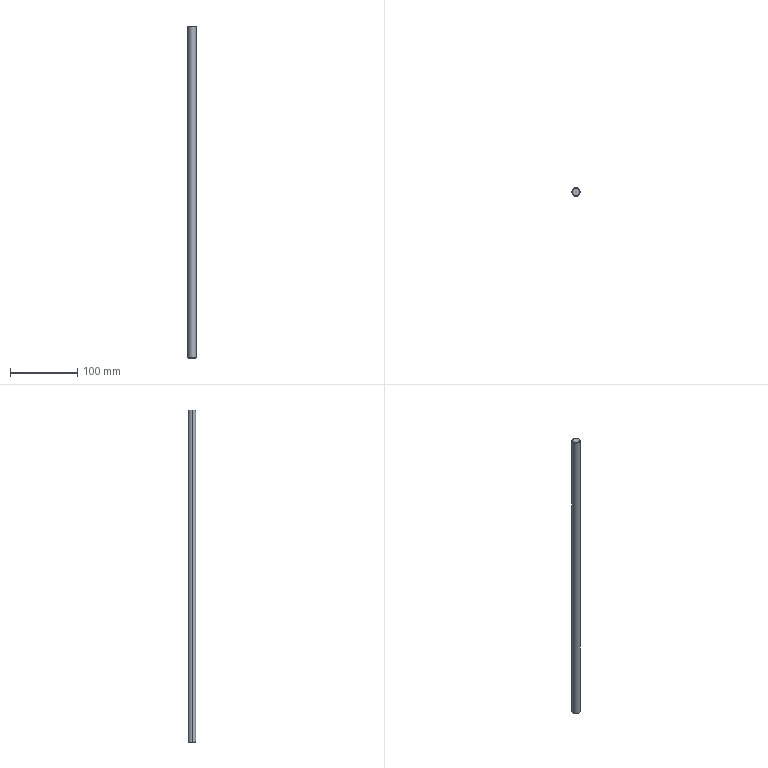Part | STEP file | 0230_011_SSFJ12-495 | 1 solid | 8 faces | box 12 x 12 x 495 mm | volume 55974 mm3 | cone 4 | cylinder 2 | plane 2 | commonest cylinder face diameters 12 x2
STEP:
#1=CARTESIAN_POINT('',(0.,0.,0.));
#2=DIRECTION('',(0.,0.,1.));
#3=DIRECTION('',(1.,0.,0.));
#4=AXIS2_PLACEMENT_3D('',#1,#2,#3);
#5=CARTESIAN_POINT('',(5.5,0.,495.));
#6=VERTEX_POINT('',#5);
#7=CARTESIAN_POINT('',(-5.5,0.,495.));
#8=VERTEX_POINT('',#7);
#9=CARTESIAN_POINT('',(0.,0.,495.));
#10=DIRECTION('',(0.,0.,1.));
#11=DIRECTION('',(1.,0.,0.));
#12=AXIS2_PLACEMENT_3D('',#9,#10,#11);
#13=CIRCLE('',#12,5.5);
#14=CARTESIAN_POINT('',(0.,0.,495.));
#15=DIRECTION('',(0.,0.,-1.));
#16=DIRECTION('',(-1.,0.,0.));
#17=AXIS2_PLACEMENT_3D('',#14,#15,#16);
#18=CONICAL_SURFACE('',#17,5.5,0.7854);
#19=CARTESIAN_POINT('',(3.142,0.));
#20=DIRECTION('',(-1.,0.));
#21=VECTOR('',#20,1.);
#22=LINE('',#19,#21);
#23=(GEOMETRIC_REPRESENTATION_CONTEXT(2)PARAMETRIC_REPRESENTATION_CONTEXT()REPRESENTATION_CONTEXT('',''));
#24=DEFINITIONAL_REPRESENTATION('',(#22),#23);
#25=PCURVE('',#18,#24);
#26=CARTESIAN_POINT('',(0.,0.,495.));
#27=DIRECTION('',(0.,0.,1.));
#28=DIRECTION('',(1.,0.,0.));
#29=AXIS2_PLACEMENT_3D('',#26,#27,#28);
#30=PLANE('',#29);
#31=CARTESIAN_POINT('',(0.,0.));
#32=DIRECTION('',(1.,0.));
#33=AXIS2_PLACEMENT_2D('',#31,#32);
#34=CIRCLE('',#33,5.5);
#35=(GEOMETRIC_REPRESENTATION_CONTEXT(2)PARAMETRIC_REPRESENTATION_CONTEXT()REPRESENTATION_CONTEXT('',''));
#36=DEFINITIONAL_REPRESENTATION('',(#34),#35);
#37=PCURVE('',#30,#36);
#38=SURFACE_CURVE('',#13,(#25,#37),.PCURVE_S1.);
#39=EDGE_CURVE('',#6,#8,#38,.T.);
#40=ORIENTED_EDGE('',*,*,#39,.F.);
#41=CARTESIAN_POINT('',(6.,0.,494.5));
#42=VERTEX_POINT('',#41);
#43=CARTESIAN_POINT('',(5.5,0.,495.));
#44=DIRECTION('',(0.7071,0.,-0.7071));
#45=VECTOR('',#44,1.);
#46=LINE('',#43,#45);
#47=CARTESIAN_POINT('',(3.142,0.));
#48=DIRECTION('',(0.,1.));
#49=VECTOR('',#48,1.);
#50=LINE('',#47,#49);
#51=(GEOMETRIC_REPRESENTATION_CONTEXT(2)PARAMETRIC_REPRESENTATION_CONTEXT()REPRESENTATION_CONTEXT('',''));
#52=DEFINITIONAL_REPRESENTATION('',(#50),#51);
#53=PCURVE('',#18,#52);
#54=CARTESIAN_POINT('',(0.,0.,495.));
#55=DIRECTION('',(0.,0.,-1.));
#56=DIRECTION('',(-1.,0.,0.));
#57=AXIS2_PLACEMENT_3D('',#54,#55,#56);
#58=CONICAL_SURFACE('',#57,5.5,0.7854);
#59=CARTESIAN_POINT('',(3.142,0.));
#60=DIRECTION('',(0.,1.));
#61=VECTOR('',#60,1.);
#62=LINE('',#59,#61);
#63=(GEOMETRIC_REPRESENTATION_CONTEXT(2)PARAMETRIC_REPRESENTATION_CONTEXT()REPRESENTATION_CONTEXT('',''));
#64=DEFINITIONAL_REPRESENTATION('',(#62),#63);
#65=PCURVE('',#58,#64);
#66=SURFACE_CURVE('',#46,(#53,#65),.PCURVE_S1.);
#67=EDGE_CURVE('',#6,#42,#66,.T.);
#68=ORIENTED_EDGE('',*,*,#67,.T.);
#69=CARTESIAN_POINT('',(-6.,0.,494.5));
#70=VERTEX_POINT('',#69);
#71=CARTESIAN_POINT('',(0.,0.,494.5));
#72=DIRECTION('',(0.,0.,-1.));
#73=DIRECTION('',(1.,0.,0.));
#74=AXIS2_PLACEMENT_3D('',#71,#72,#73);
#75=CIRCLE('',#74,6.);
#76=CARTESIAN_POINT('',(-3.142,0.5));
#77=DIRECTION('',(1.,0.));
#78=VECTOR('',#77,1.);
#79=LINE('',#76,#78);
#80=(GEOMETRIC_REPRESENTATION_CONTEXT(2)PARAMETRIC_REPRESENTATION_CONTEXT()REPRESENTATION_CONTEXT('',''));
#81=DEFINITIONAL_REPRESENTATION('',(#79),#80);
#82=PCURVE('',#18,#81);
#83=CARTESIAN_POINT('',(0.,0.,495.));
#84=DIRECTION('',(0.,0.,-1.));
#85=DIRECTION('',(-1.,0.,0.));
#86=AXIS2_PLACEMENT_3D('',#83,#84,#85);
#87=CYLINDRICAL_SURFACE('',#86,6.);
#88=CARTESIAN_POINT('',(-3.142,0.5));
#89=DIRECTION('',(1.,0.));
#90=VECTOR('',#89,1.);
#91=LINE('',#88,#90);
#92=(GEOMETRIC_REPRESENTATION_CONTEXT(2)PARAMETRIC_REPRESENTATION_CONTEXT()REPRESENTATION_CONTEXT('',''));
#93=DEFINITIONAL_REPRESENTATION('',(#91),#92);
#94=PCURVE('',#87,#93);
#95=SURFACE_CURVE('',#75,(#82,#94),.PCURVE_S1.);
#96=EDGE_CURVE('',#70,#42,#95,.T.);
#97=ORIENTED_EDGE('',*,*,#96,.F.);
#98=CARTESIAN_POINT('',(-5.5,0.,495.));
#99=DIRECTION('',(-0.7071,0.,-0.7071));
#100=VECTOR('',#99,1.);
#101=LINE('',#98,#100);
#102=CARTESIAN_POINT('',(0.,0.));
#103=DIRECTION('',(0.,1.));
#104=VECTOR('',#103,1.);
#105=LINE('',#102,#104);
#106=(GEOMETRIC_REPRESENTATION_CONTEXT(2)PARAMETRIC_REPRESENTATION_CONTEXT()REPRESENTATION_CONTEXT('',''));
#107=DEFINITIONAL_REPRESENTATION('',(#105),#106);
#108=PCURVE('',#18,#107);
#109=CARTESIAN_POINT('',(6.283,0.));
#110=DIRECTION('',(0.,1.));
#111=VECTOR('',#110,1.);
#112=LINE('',#109,#111);
#113=(GEOMETRIC_REPRESENTATION_CONTEXT(2)PARAMETRIC_REPRESENTATION_CONTEXT()REPRESENTATION_CONTEXT('',''));
#114=DEFINITIONAL_REPRESENTATION('',(#112),#113);
#115=PCURVE('',#58,#114);
#116=SURFACE_CURVE('',#101,(#108,#115),.PCURVE_S1.);
#117=EDGE_CURVE('',#8,#70,#116,.T.);
#118=ORIENTED_EDGE('',*,*,#117,.F.);
#119=EDGE_LOOP('',(#40,#68,#97,#118));
#120=FACE_BOUND('',#119,.T.);
#121=ADVANCED_FACE('',(#120),#18,.T.);
#122=CARTESIAN_POINT('',(-5.5,0.,0.));
#123=VERTEX_POINT('',#122);
#124=CARTESIAN_POINT('',(5.5,0.,0.));
#125=VERTEX_POINT('',#124);
#126=CARTESIAN_POINT('',(0.,0.,0.));
#127=DIRECTION('',(0.,0.,-1.));
#128=DIRECTION('',(1.,0.,0.));
#129=AXIS2_PLACEMENT_3D('',#126,#127,#128);
#130=CIRCLE('',#129,5.5);
#131=CARTESIAN_POINT('',(0.,0.,0.5));
#132=DIRECTION('',(0.,0.,1.));
#133=DIRECTION('',(1.,0.,0.));
#134=AXIS2_PLACEMENT_3D('',#131,#132,#133);
#135=CONICAL_SURFACE('',#134,6.,0.7854);
#136=CARTESIAN_POINT('',(6.283,-0.5));
#137=DIRECTION('',(-1.,0.));
#138=VECTOR('',#137,1.);
#139=LINE('',#136,#138);
#140=(GEOMETRIC_REPRESENTATION_CONTEXT(2)PARAMETRIC_REPRESENTATION_CONTEXT()REPRESENTATION_CONTEXT('',''));
#141=DEFINITIONAL_REPRESENTATION('',(#139),#140);
#142=PCURVE('',#135,#141);
#143=CARTESIAN_POINT('',(0.,0.,0.));
#144=DIRECTION('',(0.,0.,1.));
#145=DIRECTION('',(1.,0.,0.));
#146=AXIS2_PLACEMENT_3D('',#143,#144,#145);
#147=PLANE('',#146);
#148=CARTESIAN_POINT('',(5.5,0.));
#149=CARTESIAN_POINT('',(5.5,-9.526));
#150=CARTESIAN_POINT('',(-2.75,-4.763));
#151=CARTESIAN_POINT('',(-11.,0.));
#152=CARTESIAN_POINT('',(-2.75,4.763));
#153=CARTESIAN_POINT('',(5.5,9.526));
#154=CARTESIAN_POINT('',(5.5,0.));
#155=(BOUNDED_CURVE()B_SPLINE_CURVE(2,(#148,#149,#150,#151,#152,#153,#154),.UNSPECIFIED.,.T.,.F.)B_SPLINE_CURVE_WITH_KNOTS((1,2,2,2,2,1),(-2.094,0.,2.094,4.189,6.283,8.378),.UNSPECIFIED.)CURVE()GEOMETRIC_REPRESENTATION_ITEM()RATIONAL_B_SPLINE_CURVE((1.,0.5,1.,0.5,1.,0.5,1.))REPRESENTATION_ITEM(''));
#156=(GEOMETRIC_REPRESENTATION_CONTEXT(2)PARAMETRIC_REPRESENTATION_CONTEXT()REPRESENTATION_CONTEXT('',''));
#157=DEFINITIONAL_REPRESENTATION('',(#155),#156);
#158=PCURVE('',#147,#157);
#159=SURFACE_CURVE('',#130,(#142,#158),.PCURVE_S1.);
#160=EDGE_CURVE('',#123,#125,#159,.T.);
#161=ORIENTED_EDGE('',*,*,#160,.F.);
#162=CARTESIAN_POINT('',(-6.,0.,0.5));
#163=VERTEX_POINT('',#162);
#164=CARTESIAN_POINT('',(-6.,0.,0.5));
#165=DIRECTION('',(-0.7071,0.,0.7071));
#166=VECTOR('',#165,1.);
#167=LINE('',#164,#166);
#168=CARTESIAN_POINT('',(3.142,0.));
#169=DIRECTION('',(0.,1.));
#170=VECTOR('',#169,1.);
#171=LINE('',#168,#170);
#172=(GEOMETRIC_REPRESENTATION_CONTEXT(2)PARAMETRIC_REPRESENTATION_CONTEXT()REPRESENTATION_CONTEXT('',''));
#173=DEFINITIONAL_REPRESENTATION('',(#171),#172);
#174=PCURVE('',#135,#173);
#175=CARTESIAN_POINT('',(0.,0.,0.5));
#176=DIRECTION('',(0.,0.,1.));
#177=DIRECTION('',(1.,0.,0.));
#178=AXIS2_PLACEMENT_3D('',#175,#176,#177);
#179=CONICAL_SURFACE('',#178,6.,0.7854);
#180=CARTESIAN_POINT('',(3.142,0.));
#181=DIRECTION('',(0.,1.));
#182=VECTOR('',#181,1.);
#183=LINE('',#180,#182);
#184=(GEOMETRIC_REPRESENTATION_CONTEXT(2)PARAMETRIC_REPRESENTATION_CONTEXT()REPRESENTATION_CONTEXT('',''));
#185=DEFINITIONAL_REPRESENTATION('',(#183),#184);
#186=PCURVE('',#179,#185);
#187=SURFACE_CURVE('',#167,(#174,#186),.PCURVE_S1.);
#188=EDGE_CURVE('',#123,#163,#187,.T.);
#189=ORIENTED_EDGE('',*,*,#188,.T.);
#190=CARTESIAN_POINT('',(6.,0.,0.5));
#191=VERTEX_POINT('',#190);
#192=CARTESIAN_POINT('',(0.,0.,0.5));
#193=DIRECTION('',(0.,0.,1.));
#194=DIRECTION('',(1.,0.,0.));
#195=AXIS2_PLACEMENT_3D('',#192,#193,#194);
#196=CIRCLE('',#195,6.);
#197=CARTESIAN_POINT('',(0.,0.));
#198=DIRECTION('',(1.,0.));
#199=VECTOR('',#198,1.);
#200=LINE('',#197,#199);
#201=(GEOMETRIC_REPRESENTATION_CONTEXT(2)PARAMETRIC_REPRESENTATION_CONTEXT()REPRESENTATION_CONTEXT('',''));
#202=DEFINITIONAL_REPRESENTATION('',(#200),#201);
#203=PCURVE('',#135,#202);
#204=CARTESIAN_POINT('',(3.142,494.5));
#205=DIRECTION('',(-1.,0.));
#206=VECTOR('',#205,1.);
#207=LINE('',#204,#206);
#208=(GEOMETRIC_REPRESENTATION_CONTEXT(2)PARAMETRIC_REPRESENTATION_CONTEXT()REPRESENTATION_CONTEXT('',''));
#209=DEFINITIONAL_REPRESENTATION('',(#207),#208);
#210=PCURVE('',#87,#209);
#211=SURFACE_CURVE('',#196,(#203,#210),.PCURVE_S1.);
#212=EDGE_CURVE('',#191,#163,#211,.T.);
#213=ORIENTED_EDGE('',*,*,#212,.F.);
#214=CARTESIAN_POINT('',(6.,0.,0.5));
#215=DIRECTION('',(0.7071,0.,0.7071));
#216=VECTOR('',#215,1.);
#217=LINE('',#214,#216);
#218=CARTESIAN_POINT('',(0.,0.));
#219=DIRECTION('',(0.,1.));
#220=VECTOR('',#219,1.);
#221=LINE('',#218,#220);
#222=(GEOMETRIC_REPRESENTATION_CONTEXT(2)PARAMETRIC_REPRESENTATION_CONTEXT()REPRESENTATION_CONTEXT('',''));
#223=DEFINITIONAL_REPRESENTATION('',(#221),#222);
#224=PCURVE('',#135,#223);
#225=CARTESIAN_POINT('',(6.283,0.));
#226=DIRECTION('',(0.,1.));
#227=VECTOR('',#226,1.);
#228=LINE('',#225,#227);
#229=(GEOMETRIC_REPRESENTATION_CONTEXT(2)PARAMETRIC_REPRESENTATION_CONTEXT()REPRESENTATION_CONTEXT('',''));
#230=DEFINITIONAL_REPRESENTATION('',(#228),#229);
#231=PCURVE('',#179,#230);
#232=SURFACE_CURVE('',#217,(#224,#231),.PCURVE_S1.);
#233=EDGE_CURVE('',#125,#191,#232,.T.);
#234=ORIENTED_EDGE('',*,*,#233,.F.);
#235=EDGE_LOOP('',(#161,#189,#213,#234));
#236=FACE_BOUND('',#235,.T.);
#237=ADVANCED_FACE('',(#236),#135,.T.);
#238=ORIENTED_EDGE('',*,*,#96,.T.);
#239=CARTESIAN_POINT('',(6.,0.,495.));
#240=DIRECTION('',(0.,0.,-1.));
#241=VECTOR('',#240,1.);
#242=LINE('',#239,#241);
#243=CARTESIAN_POINT('',(3.142,0.));
#244=DIRECTION('',(0.,1.));
#245=VECTOR('',#244,1.);
#246=LINE('',#243,#245);
#247=(GEOMETRIC_REPRESENTATION_CONTEXT(2)PARAMETRIC_REPRESENTATION_CONTEXT()REPRESENTATION_CONTEXT('',''));
#248=DEFINITIONAL_REPRESENTATION('',(#246),#247);
#249=PCURVE('',#87,#248);
#250=CARTESIAN_POINT('',(0.,0.,495.));
#251=DIRECTION('',(0.,0.,-1.));
#252=DIRECTION('',(-1.,0.,0.));
#253=AXIS2_PLACEMENT_3D('',#250,#251,#252);
#254=CYLINDRICAL_SURFACE('',#253,6.);
#255=CARTESIAN_POINT('',(3.142,0.));
#256=DIRECTION('',(0.,1.));
#257=VECTOR('',#256,1.);
#258=LINE('',#255,#257);
#259=(GEOMETRIC_REPRESENTATION_CONTEXT(2)PARAMETRIC_REPRESENTATION_CONTEXT()REPRESENTATION_CONTEXT('',''));
#260=DEFINITIONAL_REPRESENTATION('',(#258),#259);
#261=PCURVE('',#254,#260);
#262=SURFACE_CURVE('',#242,(#249,#261),.PCURVE_S1.);
#263=EDGE_CURVE('',#42,#191,#262,.T.);
#264=ORIENTED_EDGE('',*,*,#263,.T.);
#265=ORIENTED_EDGE('',*,*,#212,.T.);
#266=CARTESIAN_POINT('',(-6.,0.,495.));
#267=DIRECTION('',(0.,0.,-1.));
#268=VECTOR('',#267,1.);
#269=LINE('',#266,#268);
#270=CARTESIAN_POINT('',(0.,0.));
#271=DIRECTION('',(0.,1.));
#272=VECTOR('',#271,1.);
#273=LINE('',#270,#272);
#274=(GEOMETRIC_REPRESENTATION_CONTEXT(2)PARAMETRIC_REPRESENTATION_CONTEXT()REPRESENTATION_CONTEXT('',''));
#275=DEFINITIONAL_REPRESENTATION('',(#273),#274);
#276=PCURVE('',#87,#275);
#277=CARTESIAN_POINT('',(6.283,0.));
#278=DIRECTION('',(0.,1.));
#279=VECTOR('',#278,1.);
#280=LINE('',#277,#279);
#281=(GEOMETRIC_REPRESENTATION_CONTEXT(2)PARAMETRIC_REPRESENTATION_CONTEXT()REPRESENTATION_CONTEXT('',''));
#282=DEFINITIONAL_REPRESENTATION('',(#280),#281);
#283=PCURVE('',#254,#282);
#284=SURFACE_CURVE('',#269,(#276,#283),.PCURVE_S1.);
#285=EDGE_CURVE('',#70,#163,#284,.T.);
#286=ORIENTED_EDGE('',*,*,#285,.F.);
#287=EDGE_LOOP('',(#238,#264,#265,#286));
#288=FACE_BOUND('',#287,.T.);
#289=ADVANCED_FACE('',(#288),#87,.T.);
#290=ORIENTED_EDGE('',*,*,#263,.F.);
#291=CARTESIAN_POINT('',(0.,0.,494.5));
#292=DIRECTION('',(0.,0.,-1.));
#293=DIRECTION('',(1.,0.,0.));
#294=AXIS2_PLACEMENT_3D('',#291,#292,#293);
#295=CIRCLE('',#294,6.);
#296=CARTESIAN_POINT('',(3.142,0.5));
#297=DIRECTION('',(1.,0.));
#298=VECTOR('',#297,1.);
#299=LINE('',#296,#298);
#300=(GEOMETRIC_REPRESENTATION_CONTEXT(2)PARAMETRIC_REPRESENTATION_CONTEXT()REPRESENTATION_CONTEXT('',''));
#301=DEFINITIONAL_REPRESENTATION('',(#299),#300);
#302=PCURVE('',#254,#301);
#303=CARTESIAN_POINT('',(3.142,0.5));
#304=DIRECTION('',(1.,0.));
#305=VECTOR('',#304,1.);
#306=LINE('',#303,#305);
#307=(GEOMETRIC_REPRESENTATION_CONTEXT(2)PARAMETRIC_REPRESENTATION_CONTEXT()REPRESENTATION_CONTEXT('',''));
#308=DEFINITIONAL_REPRESENTATION('',(#306),#307);
#309=PCURVE('',#58,#308);
#310=SURFACE_CURVE('',#295,(#302,#309),.PCURVE_S1.);
#311=EDGE_CURVE('',#42,#70,#310,.T.);
#312=ORIENTED_EDGE('',*,*,#311,.T.);
#313=ORIENTED_EDGE('',*,*,#285,.T.);
#314=CARTESIAN_POINT('',(0.,0.,0.5));
#315=DIRECTION('',(0.,0.,1.));
#316=DIRECTION('',(1.,0.,0.));
#317=AXIS2_PLACEMENT_3D('',#314,#315,#316);
#318=CIRCLE('',#317,6.);
#319=CARTESIAN_POINT('',(9.425,494.5));
#320=DIRECTION('',(-1.,0.));
#321=VECTOR('',#320,1.);
#322=LINE('',#319,#321);
#323=(GEOMETRIC_REPRESENTATION_CONTEXT(2)PARAMETRIC_REPRESENTATION_CONTEXT()REPRESENTATION_CONTEXT('',''));
#324=DEFINITIONAL_REPRESENTATION('',(#322),#323);
#325=PCURVE('',#254,#324);
#326=CARTESIAN_POINT('',(0.,0.));
#327=DIRECTION('',(1.,0.));
#328=VECTOR('',#327,1.);
#329=LINE('',#326,#328);
#330=(GEOMETRIC_REPRESENTATION_CONTEXT(2)PARAMETRIC_REPRESENTATION_CONTEXT()REPRESENTATION_CONTEXT('',''));
#331=DEFINITIONAL_REPRESENTATION('',(#329),#330);
#332=PCURVE('',#179,#331);
#333=SURFACE_CURVE('',#318,(#325,#332),.PCURVE_S1.);
#334=EDGE_CURVE('',#163,#191,#333,.T.);
#335=ORIENTED_EDGE('',*,*,#334,.T.);
#336=EDGE_LOOP('',(#290,#312,#313,#335));
#337=FACE_BOUND('',#336,.T.);
#338=ADVANCED_FACE('',(#337),#254,.T.);
#339=CARTESIAN_POINT('',(0.,0.,495.));
#340=DIRECTION('',(0.,0.,1.));
#341=DIRECTION('',(1.,0.,0.));
#342=AXIS2_PLACEMENT_3D('',#339,#340,#341);
#343=CIRCLE('',#342,5.5);
#344=CARTESIAN_POINT('',(0.,0.));
#345=DIRECTION('',(1.,0.));
#346=AXIS2_PLACEMENT_2D('',#344,#345);
#347=CIRCLE('',#346,5.5);
#348=(GEOMETRIC_REPRESENTATION_CONTEXT(2)PARAMETRIC_REPRESENTATION_CONTEXT()REPRESENTATION_CONTEXT('',''));
#349=DEFINITIONAL_REPRESENTATION('',(#347),#348);
#350=PCURVE('',#30,#349);
#351=CARTESIAN_POINT('',(9.425,0.));
#352=DIRECTION('',(-1.,0.));
#353=VECTOR('',#352,1.);
#354=LINE('',#351,#353);
#355=(GEOMETRIC_REPRESENTATION_CONTEXT(2)PARAMETRIC_REPRESENTATION_CONTEXT()REPRESENTATION_CONTEXT('',''));
#356=DEFINITIONAL_REPRESENTATION('',(#354),#355);
#357=PCURVE('',#58,#356);
#358=SURFACE_CURVE('',#343,(#350,#357),.PCURVE_S1.);
#359=EDGE_CURVE('',#8,#6,#358,.T.);
#360=ORIENTED_EDGE('',*,*,#359,.T.);
#361=ORIENTED_EDGE('',*,*,#39,.T.);
#362=EDGE_LOOP('',(#360,#361));
#363=FACE_BOUND('',#362,.T.);
#364=ADVANCED_FACE('',(#363),#30,.T.);
#365=CARTESIAN_POINT('',(0.,0.,0.));
#366=DIRECTION('',(0.,0.,-1.));
#367=DIRECTION('',(1.,0.,0.));
#368=AXIS2_PLACEMENT_3D('',#365,#366,#367);
#369=CIRCLE('',#368,5.5);
#370=CARTESIAN_POINT('',(5.5,0.));
#371=CARTESIAN_POINT('',(5.5,-9.526));
#372=CARTESIAN_POINT('',(-2.75,-4.763));
#373=CARTESIAN_POINT('',(-11.,0.));
#374=CARTESIAN_POINT('',(-2.75,4.763));
#375=CARTESIAN_POINT('',(5.5,9.526));
#376=CARTESIAN_POINT('',(5.5,0.));
#377=(BOUNDED_CURVE()B_SPLINE_CURVE(2,(#370,#371,#372,#373,#374,#375,#376),.UNSPECIFIED.,.T.,.F.)B_SPLINE_CURVE_WITH_KNOTS((1,2,2,2,2,1),(-2.094,0.,2.094,4.189,6.283,8.378),.UNSPECIFIED.)CURVE()GEOMETRIC_REPRESENTATION_ITEM()RATIONAL_B_SPLINE_CURVE((1.,0.5,1.,0.5,1.,0.5,1.))REPRESENTATION_ITEM(''));
#378=(GEOMETRIC_REPRESENTATION_CONTEXT(2)PARAMETRIC_REPRESENTATION_CONTEXT()REPRESENTATION_CONTEXT('',''));
#379=DEFINITIONAL_REPRESENTATION('',(#377),#378);
#380=PCURVE('',#147,#379);
#381=CARTESIAN_POINT('',(6.283,-0.5));
#382=DIRECTION('',(-1.,0.));
#383=VECTOR('',#382,1.);
#384=LINE('',#381,#383);
#385=(GEOMETRIC_REPRESENTATION_CONTEXT(2)PARAMETRIC_REPRESENTATION_CONTEXT()REPRESENTATION_CONTEXT('',''));
#386=DEFINITIONAL_REPRESENTATION('',(#384),#385);
#387=PCURVE('',#179,#386);
#388=SURFACE_CURVE('',#369,(#380,#387),.PCURVE_S1.);
#389=EDGE_CURVE('',#125,#123,#388,.T.);
#390=ORIENTED_EDGE('',*,*,#389,.T.);
#391=ORIENTED_EDGE('',*,*,#160,.T.);
#392=EDGE_LOOP('',(#390,#391));
#393=FACE_BOUND('',#392,.T.);
#394=ADVANCED_FACE('',(#393),#147,.F.);
#395=ORIENTED_EDGE('',*,*,#188,.F.);
#396=ORIENTED_EDGE('',*,*,#389,.F.);
#397=ORIENTED_EDGE('',*,*,#233,.T.);
#398=ORIENTED_EDGE('',*,*,#334,.F.);
#399=EDGE_LOOP('',(#395,#396,#397,#398));
#400=FACE_BOUND('',#399,.T.);
#401=ADVANCED_FACE('',(#400),#179,.T.);
#402=ORIENTED_EDGE('',*,*,#67,.F.);
#403=ORIENTED_EDGE('',*,*,#359,.F.);
#404=ORIENTED_EDGE('',*,*,#117,.T.);
#405=ORIENTED_EDGE('',*,*,#311,.F.);
#406=EDGE_LOOP('',(#402,#403,#404,#405));
#407=FACE_BOUND('',#406,.T.);
#408=ADVANCED_FACE('',(#407),#58,.T.);
#409=CLOSED_SHELL('',(#121,#237,#289,#338,#364,#394,#401,#408));
#410=MANIFOLD_SOLID_BREP('',#409);
#411=(LENGTH_UNIT()NAMED_UNIT(*)SI_UNIT(.MILLI.,.METRE.));
#412=UNCERTAINTY_MEASURE_WITH_UNIT(LENGTH_MEASURE(0.0000001),#411,'','');
#413=(NAMED_UNIT(*)PLANE_ANGLE_UNIT()SI_UNIT($,.RADIAN.));
#414=(NAMED_UNIT(*)SI_UNIT($,.STERADIAN.)SOLID_ANGLE_UNIT());
#415=(GEOMETRIC_REPRESENTATION_CONTEXT(3)GLOBAL_UNCERTAINTY_ASSIGNED_CONTEXT((#412))GLOBAL_UNIT_ASSIGNED_CONTEXT((#411,#413,#414))REPRESENTATION_CONTEXT('',''));
#416=ADVANCED_BREP_SHAPE_REPRESENTATION('',(#4,#410),#415);